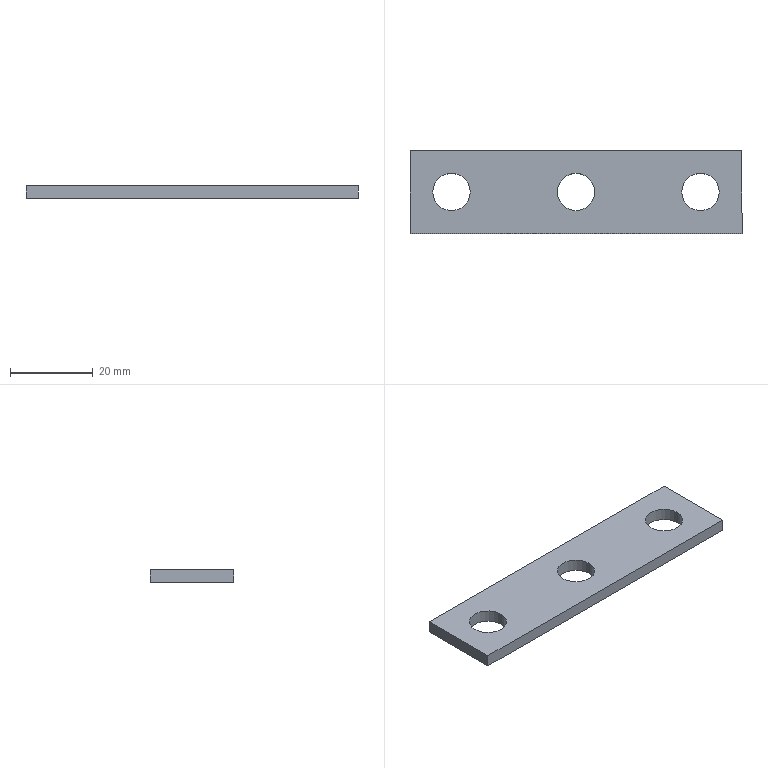Part | SolidWorks | features BaseBody 1 | 1 solid | 12 faces | box 80 x 20 x 3 mm | volume 4227 mm3 | cylinder 6 | plane 6 | commonest cylinder face diameters 9 x6
STEP:
#1=CARTESIAN_POINT('',(-34.5,0.,-3.));
#2=VERTEX_POINT('',#1);
#3=CARTESIAN_POINT('',(-34.5,0.,0.));
#4=VERTEX_POINT('',#3);
#5=CARTESIAN_POINT('',(-34.5,0.,-10.));
#6=DIRECTION('',(0.,0.,1.));
#7=VECTOR('',#6,1000.);
#8=LINE('',#5,#7);
#9=EDGE_CURVE('',#2,#4,#8,.T.);
#10=ORIENTED_EDGE('',*,*,#9,.F.);
#11=CARTESIAN_POINT('',(-25.5,0.,-3.));
#12=VERTEX_POINT('',#11);
#13=CARTESIAN_POINT('',(-30.,0.,-3.));
#14=DIRECTION('',(0.,0.,1.));
#15=DIRECTION('',(1.,0.,0.));
#16=AXIS2_PLACEMENT_3D('',#13,#14,#15);
#17=CIRCLE('',#16,4.5);
#18=EDGE_CURVE('',#12,#2,#17,.T.);
#19=ORIENTED_EDGE('',*,*,#18,.F.);
#20=CARTESIAN_POINT('',(-25.5,0.,0.));
#21=VERTEX_POINT('',#20);
#22=CARTESIAN_POINT('',(-25.5,0.,-10.));
#23=DIRECTION('',(0.,0.,1.));
#24=VECTOR('',#23,1000.);
#25=LINE('',#22,#24);
#26=EDGE_CURVE('',#12,#21,#25,.T.);
#27=ORIENTED_EDGE('',*,*,#26,.T.);
#28=CARTESIAN_POINT('',(-30.,0.,0.));
#29=DIRECTION('',(0.,0.,1.));
#30=DIRECTION('',(-1.,0.,0.));
#31=AXIS2_PLACEMENT_3D('',#28,#29,#30);
#32=CIRCLE('',#31,4.5);
#33=EDGE_CURVE('',#21,#4,#32,.T.);
#34=ORIENTED_EDGE('',*,*,#33,.T.);
#35=EDGE_LOOP('',(#10,#19,#27,#34));
#36=FACE_OUTER_BOUND('',#35,.T.);
#37=CARTESIAN_POINT('',(-30.,0.,-10.));
#38=DIRECTION('',(0.,0.,1.));
#39=DIRECTION('',(1.,0.,0.));
#40=AXIS2_PLACEMENT_3D('',#37,#38,#39);
#41=CYLINDRICAL_SURFACE('',#40,4.5);
#42=ADVANCED_FACE('',(#36),#41,.F.);
#43=CARTESIAN_POINT('',(25.5,0.,-3.));
#44=VERTEX_POINT('',#43);
#45=CARTESIAN_POINT('',(25.5,0.,0.));
#46=VERTEX_POINT('',#45);
#47=CARTESIAN_POINT('',(25.5,0.,-10.));
#48=DIRECTION('',(0.,0.,1.));
#49=VECTOR('',#48,1000.);
#50=LINE('',#47,#49);
#51=EDGE_CURVE('',#44,#46,#50,.T.);
#52=ORIENTED_EDGE('',*,*,#51,.F.);
#53=CARTESIAN_POINT('',(34.5,0.,-3.));
#54=VERTEX_POINT('',#53);
#55=CARTESIAN_POINT('',(30.,0.,-3.));
#56=DIRECTION('',(0.,0.,1.));
#57=DIRECTION('',(1.,0.,0.));
#58=AXIS2_PLACEMENT_3D('',#55,#56,#57);
#59=CIRCLE('',#58,4.5);
#60=EDGE_CURVE('',#54,#44,#59,.T.);
#61=ORIENTED_EDGE('',*,*,#60,.F.);
#62=CARTESIAN_POINT('',(34.5,0.,0.));
#63=VERTEX_POINT('',#62);
#64=CARTESIAN_POINT('',(34.5,0.,-10.));
#65=DIRECTION('',(0.,0.,1.));
#66=VECTOR('',#65,1000.);
#67=LINE('',#64,#66);
#68=EDGE_CURVE('',#54,#63,#67,.T.);
#69=ORIENTED_EDGE('',*,*,#68,.T.);
#70=CARTESIAN_POINT('',(30.,0.,0.));
#71=DIRECTION('',(0.,0.,1.));
#72=DIRECTION('',(1.,0.,0.));
#73=AXIS2_PLACEMENT_3D('',#70,#71,#72);
#74=CIRCLE('',#73,4.5);
#75=EDGE_CURVE('',#63,#46,#74,.T.);
#76=ORIENTED_EDGE('',*,*,#75,.T.);
#77=EDGE_LOOP('',(#52,#61,#69,#76));
#78=FACE_OUTER_BOUND('',#77,.T.);
#79=CARTESIAN_POINT('',(30.,0.,-10.));
#80=DIRECTION('',(0.,0.,1.));
#81=DIRECTION('',(1.,0.,0.));
#82=AXIS2_PLACEMENT_3D('',#79,#80,#81);
#83=CYLINDRICAL_SURFACE('',#82,4.5);
#84=ADVANCED_FACE('',(#78),#83,.F.);
#85=CARTESIAN_POINT('',(-4.5,0.,-3.));
#86=VERTEX_POINT('',#85);
#87=CARTESIAN_POINT('',(-4.5,0.,0.));
#88=VERTEX_POINT('',#87);
#89=CARTESIAN_POINT('',(-4.5,0.,-10.));
#90=DIRECTION('',(0.,0.,1.));
#91=VECTOR('',#90,1000.);
#92=LINE('',#89,#91);
#93=EDGE_CURVE('',#86,#88,#92,.T.);
#94=ORIENTED_EDGE('',*,*,#93,.F.);
#95=CARTESIAN_POINT('',(4.5,0.,-3.));
#96=VERTEX_POINT('',#95);
#97=CARTESIAN_POINT('',(0.,0.,-3.));
#98=DIRECTION('',(0.,0.,1.));
#99=DIRECTION('',(1.,0.,0.));
#100=AXIS2_PLACEMENT_3D('',#97,#98,#99);
#101=CIRCLE('',#100,4.5);
#102=EDGE_CURVE('',#96,#86,#101,.T.);
#103=ORIENTED_EDGE('',*,*,#102,.F.);
#104=CARTESIAN_POINT('',(4.5,0.,0.));
#105=VERTEX_POINT('',#104);
#106=CARTESIAN_POINT('',(4.5,0.,-10.));
#107=DIRECTION('',(0.,0.,1.));
#108=VECTOR('',#107,1000.);
#109=LINE('',#106,#108);
#110=EDGE_CURVE('',#96,#105,#109,.T.);
#111=ORIENTED_EDGE('',*,*,#110,.T.);
#112=CARTESIAN_POINT('',(0.,0.,0.));
#113=DIRECTION('',(0.,0.,1.));
#114=DIRECTION('',(1.,0.,0.));
#115=AXIS2_PLACEMENT_3D('',#112,#113,#114);
#116=CIRCLE('',#115,4.5);
#117=EDGE_CURVE('',#105,#88,#116,.T.);
#118=ORIENTED_EDGE('',*,*,#117,.T.);
#119=EDGE_LOOP('',(#94,#103,#111,#118));
#120=FACE_OUTER_BOUND('',#119,.T.);
#121=CARTESIAN_POINT('',(0.,0.,-10.));
#122=DIRECTION('',(0.,0.,1.));
#123=DIRECTION('',(1.,0.,0.));
#124=AXIS2_PLACEMENT_3D('',#121,#122,#123);
#125=CYLINDRICAL_SURFACE('',#124,4.5);
#126=ADVANCED_FACE('',(#120),#125,.F.);
#127=ORIENTED_EDGE('',*,*,#117,.F.);
#128=CARTESIAN_POINT('',(0.,0.,0.));
#129=DIRECTION('',(0.,0.,1.));
#130=DIRECTION('',(1.,0.,0.));
#131=AXIS2_PLACEMENT_3D('',#128,#129,#130);
#132=CIRCLE('',#131,4.5);
#133=EDGE_CURVE('',#88,#105,#132,.T.);
#134=ORIENTED_EDGE('',*,*,#133,.F.);
#135=EDGE_LOOP('',(#127,#134));
#136=FACE_BOUND('',#135,.T.);
#137=ORIENTED_EDGE('',*,*,#75,.F.);
#138=CARTESIAN_POINT('',(30.,0.,0.));
#139=DIRECTION('',(0.,0.,1.));
#140=DIRECTION('',(1.,0.,0.));
#141=AXIS2_PLACEMENT_3D('',#138,#139,#140);
#142=CIRCLE('',#141,4.5);
#143=EDGE_CURVE('',#46,#63,#142,.T.);
#144=ORIENTED_EDGE('',*,*,#143,.F.);
#145=EDGE_LOOP('',(#137,#144));
#146=FACE_BOUND('',#145,.T.);
#147=ORIENTED_EDGE('',*,*,#33,.F.);
#148=CARTESIAN_POINT('',(-30.,0.,0.));
#149=DIRECTION('',(0.,0.,1.));
#150=DIRECTION('',(-1.,0.,0.));
#151=AXIS2_PLACEMENT_3D('',#148,#149,#150);
#152=CIRCLE('',#151,4.5);
#153=EDGE_CURVE('',#4,#21,#152,.T.);
#154=ORIENTED_EDGE('',*,*,#153,.F.);
#155=EDGE_LOOP('',(#147,#154));
#156=FACE_BOUND('',#155,.T.);
#157=CARTESIAN_POINT('',(40.,-10.,0.));
#158=VERTEX_POINT('',#157);
#159=CARTESIAN_POINT('',(40.,10.,0.));
#160=VERTEX_POINT('',#159);
#161=CARTESIAN_POINT('',(40.,10.,0.));
#162=DIRECTION('',(0.,1.,0.));
#163=VECTOR('',#162,1000.);
#164=LINE('',#161,#163);
#165=EDGE_CURVE('',#158,#160,#164,.T.);
#166=ORIENTED_EDGE('',*,*,#165,.T.);
#167=CARTESIAN_POINT('',(-40.,10.,0.));
#168=VERTEX_POINT('',#167);
#169=CARTESIAN_POINT('',(-40.,10.,0.));
#170=DIRECTION('',(-1.,0.,0.));
#171=VECTOR('',#170,1000.);
#172=LINE('',#169,#171);
#173=EDGE_CURVE('',#160,#168,#172,.T.);
#174=ORIENTED_EDGE('',*,*,#173,.T.);
#175=CARTESIAN_POINT('',(-40.,-10.,0.));
#176=VERTEX_POINT('',#175);
#177=CARTESIAN_POINT('',(-40.,10.,0.));
#178=DIRECTION('',(0.,-1.,0.));
#179=VECTOR('',#178,1000.);
#180=LINE('',#177,#179);
#181=EDGE_CURVE('',#168,#176,#180,.T.);
#182=ORIENTED_EDGE('',*,*,#181,.T.);
#183=CARTESIAN_POINT('',(-40.,-10.,0.));
#184=DIRECTION('',(1.,0.,0.));
#185=VECTOR('',#184,1000.);
#186=LINE('',#183,#185);
#187=EDGE_CURVE('',#176,#158,#186,.T.);
#188=ORIENTED_EDGE('',*,*,#187,.T.);
#189=EDGE_LOOP('',(#166,#174,#182,#188));
#190=FACE_OUTER_BOUND('',#189,.T.);
#191=CARTESIAN_POINT('',(0.,0.,0.));
#192=DIRECTION('',(0.,0.,1.));
#193=DIRECTION('',(1.,0.,0.));
#194=AXIS2_PLACEMENT_3D('',#191,#192,#193);
#195=PLANE('',#194);
#196=ADVANCED_FACE('',(#136,#146,#156,#190),#195,.T.);
#197=ORIENTED_EDGE('',*,*,#102,.T.);
#198=CARTESIAN_POINT('',(0.,0.,-3.));
#199=DIRECTION('',(0.,0.,1.));
#200=DIRECTION('',(1.,0.,0.));
#201=AXIS2_PLACEMENT_3D('',#198,#199,#200);
#202=CIRCLE('',#201,4.5);
#203=EDGE_CURVE('',#86,#96,#202,.T.);
#204=ORIENTED_EDGE('',*,*,#203,.T.);
#205=EDGE_LOOP('',(#197,#204));
#206=FACE_BOUND('',#205,.T.);
#207=ORIENTED_EDGE('',*,*,#60,.T.);
#208=CARTESIAN_POINT('',(30.,0.,-3.));
#209=DIRECTION('',(0.,0.,1.));
#210=DIRECTION('',(1.,0.,0.));
#211=AXIS2_PLACEMENT_3D('',#208,#209,#210);
#212=CIRCLE('',#211,4.5);
#213=EDGE_CURVE('',#44,#54,#212,.T.);
#214=ORIENTED_EDGE('',*,*,#213,.T.);
#215=EDGE_LOOP('',(#207,#214));
#216=FACE_BOUND('',#215,.T.);
#217=ORIENTED_EDGE('',*,*,#18,.T.);
#218=CARTESIAN_POINT('',(-30.,0.,-3.));
#219=DIRECTION('',(0.,0.,1.));
#220=DIRECTION('',(1.,0.,0.));
#221=AXIS2_PLACEMENT_3D('',#218,#219,#220);
#222=CIRCLE('',#221,4.5);
#223=EDGE_CURVE('',#2,#12,#222,.T.);
#224=ORIENTED_EDGE('',*,*,#223,.T.);
#225=EDGE_LOOP('',(#217,#224));
#226=FACE_BOUND('',#225,.T.);
#227=CARTESIAN_POINT('',(40.,-10.,-3.));
#228=VERTEX_POINT('',#227);
#229=CARTESIAN_POINT('',(40.,10.,-3.));
#230=VERTEX_POINT('',#229);
#231=CARTESIAN_POINT('',(40.,10.,-3.));
#232=DIRECTION('',(0.,1.,0.));
#233=VECTOR('',#232,1000.);
#234=LINE('',#231,#233);
#235=EDGE_CURVE('',#228,#230,#234,.T.);
#236=ORIENTED_EDGE('',*,*,#235,.F.);
#237=CARTESIAN_POINT('',(-40.,-10.,-3.));
#238=VERTEX_POINT('',#237);
#239=CARTESIAN_POINT('',(-40.,-10.,-3.));
#240=DIRECTION('',(1.,0.,0.));
#241=VECTOR('',#240,1000.);
#242=LINE('',#239,#241);
#243=EDGE_CURVE('',#238,#228,#242,.T.);
#244=ORIENTED_EDGE('',*,*,#243,.F.);
#245=CARTESIAN_POINT('',(-40.,10.,-3.));
#246=VERTEX_POINT('',#245);
#247=CARTESIAN_POINT('',(-40.,10.,-3.));
#248=DIRECTION('',(0.,-1.,0.));
#249=VECTOR('',#248,1000.);
#250=LINE('',#247,#249);
#251=EDGE_CURVE('',#246,#238,#250,.T.);
#252=ORIENTED_EDGE('',*,*,#251,.F.);
#253=CARTESIAN_POINT('',(-40.,10.,-3.));
#254=DIRECTION('',(-1.,0.,0.));
#255=VECTOR('',#254,1000.);
#256=LINE('',#253,#255);
#257=EDGE_CURVE('',#230,#246,#256,.T.);
#258=ORIENTED_EDGE('',*,*,#257,.F.);
#259=EDGE_LOOP('',(#236,#244,#252,#258));
#260=FACE_OUTER_BOUND('',#259,.T.);
#261=CARTESIAN_POINT('',(0.,0.,-3.));
#262=DIRECTION('',(0.,0.,1.));
#263=DIRECTION('',(1.,0.,0.));
#264=AXIS2_PLACEMENT_3D('',#261,#262,#263);
#265=PLANE('',#264);
#266=ADVANCED_FACE('',(#206,#216,#226,#260),#265,.F.);
#267=ORIENTED_EDGE('',*,*,#173,.F.);
#268=CARTESIAN_POINT('',(40.,10.,-3.));
#269=DIRECTION('',(0.,0.,1.));
#270=VECTOR('',#269,1000.);
#271=LINE('',#268,#270);
#272=EDGE_CURVE('',#230,#160,#271,.T.);
#273=ORIENTED_EDGE('',*,*,#272,.F.);
#274=ORIENTED_EDGE('',*,*,#257,.T.);
#275=CARTESIAN_POINT('',(-40.,10.,-3.));
#276=DIRECTION('',(0.,0.,1.));
#277=VECTOR('',#276,1000.);
#278=LINE('',#275,#277);
#279=EDGE_CURVE('',#246,#168,#278,.T.);
#280=ORIENTED_EDGE('',*,*,#279,.T.);
#281=EDGE_LOOP('',(#267,#273,#274,#280));
#282=FACE_OUTER_BOUND('',#281,.T.);
#283=CARTESIAN_POINT('',(-40.,10.,-3.));
#284=DIRECTION('',(0.,1.,0.));
#285=DIRECTION('',(1.,0.,0.));
#286=AXIS2_PLACEMENT_3D('',#283,#284,#285);
#287=PLANE('',#286);
#288=ADVANCED_FACE('',(#282),#287,.T.);
#289=ORIENTED_EDGE('',*,*,#181,.F.);
#290=ORIENTED_EDGE('',*,*,#279,.F.);
#291=ORIENTED_EDGE('',*,*,#251,.T.);
#292=CARTESIAN_POINT('',(-40.,-10.,-3.));
#293=DIRECTION('',(0.,0.,1.));
#294=VECTOR('',#293,1000.);
#295=LINE('',#292,#294);
#296=EDGE_CURVE('',#238,#176,#295,.T.);
#297=ORIENTED_EDGE('',*,*,#296,.T.);
#298=EDGE_LOOP('',(#289,#290,#291,#297));
#299=FACE_OUTER_BOUND('',#298,.T.);
#300=CARTESIAN_POINT('',(-40.,10.,-3.));
#301=DIRECTION('',(-1.,0.,0.));
#302=DIRECTION('',(0.,0.,1.));
#303=AXIS2_PLACEMENT_3D('',#300,#301,#302);
#304=PLANE('',#303);
#305=ADVANCED_FACE('',(#299),#304,.T.);
#306=ORIENTED_EDGE('',*,*,#187,.F.);
#307=ORIENTED_EDGE('',*,*,#296,.F.);
#308=ORIENTED_EDGE('',*,*,#243,.T.);
#309=CARTESIAN_POINT('',(40.,-10.,-3.));
#310=DIRECTION('',(0.,0.,1.));
#311=VECTOR('',#310,1000.);
#312=LINE('',#309,#311);
#313=EDGE_CURVE('',#228,#158,#312,.T.);
#314=ORIENTED_EDGE('',*,*,#313,.T.);
#315=EDGE_LOOP('',(#306,#307,#308,#314));
#316=FACE_OUTER_BOUND('',#315,.T.);
#317=CARTESIAN_POINT('',(-40.,-10.,-3.));
#318=DIRECTION('',(0.,-1.,0.));
#319=DIRECTION('',(0.,0.,-1.));
#320=AXIS2_PLACEMENT_3D('',#317,#318,#319);
#321=PLANE('',#320);
#322=ADVANCED_FACE('',(#316),#321,.T.);
#323=ORIENTED_EDGE('',*,*,#165,.F.);
#324=ORIENTED_EDGE('',*,*,#313,.F.);
#325=ORIENTED_EDGE('',*,*,#235,.T.);
#326=ORIENTED_EDGE('',*,*,#272,.T.);
#327=EDGE_LOOP('',(#323,#324,#325,#326));
#328=FACE_OUTER_BOUND('',#327,.T.);
#329=CARTESIAN_POINT('',(40.,10.,-3.));
#330=DIRECTION('',(1.,0.,0.));
#331=DIRECTION('',(0.,1.,0.));
#332=AXIS2_PLACEMENT_3D('',#329,#330,#331);
#333=PLANE('',#332);
#334=ADVANCED_FACE('',(#328),#333,.T.);
#335=ORIENTED_EDGE('',*,*,#203,.F.);
#336=ORIENTED_EDGE('',*,*,#93,.T.);
#337=ORIENTED_EDGE('',*,*,#133,.T.);
#338=ORIENTED_EDGE('',*,*,#110,.F.);
#339=EDGE_LOOP('',(#335,#336,#337,#338));
#340=FACE_OUTER_BOUND('',#339,.T.);
#341=CARTESIAN_POINT('',(0.,0.,-10.));
#342=DIRECTION('',(0.,0.,1.));
#343=DIRECTION('',(1.,0.,0.));
#344=AXIS2_PLACEMENT_3D('',#341,#342,#343);
#345=CYLINDRICAL_SURFACE('',#344,4.5);
#346=ADVANCED_FACE('',(#340),#345,.F.);
#347=ORIENTED_EDGE('',*,*,#213,.F.);
#348=ORIENTED_EDGE('',*,*,#51,.T.);
#349=ORIENTED_EDGE('',*,*,#143,.T.);
#350=ORIENTED_EDGE('',*,*,#68,.F.);
#351=EDGE_LOOP('',(#347,#348,#349,#350));
#352=FACE_OUTER_BOUND('',#351,.T.);
#353=CARTESIAN_POINT('',(30.,0.,-10.));
#354=DIRECTION('',(0.,0.,1.));
#355=DIRECTION('',(1.,0.,0.));
#356=AXIS2_PLACEMENT_3D('',#353,#354,#355);
#357=CYLINDRICAL_SURFACE('',#356,4.5);
#358=ADVANCED_FACE('',(#352),#357,.F.);
#359=ORIENTED_EDGE('',*,*,#223,.F.);
#360=ORIENTED_EDGE('',*,*,#9,.T.);
#361=ORIENTED_EDGE('',*,*,#153,.T.);
#362=ORIENTED_EDGE('',*,*,#26,.F.);
#363=EDGE_LOOP('',(#359,#360,#361,#362));
#364=FACE_OUTER_BOUND('',#363,.T.);
#365=CARTESIAN_POINT('',(-30.,0.,-10.));
#366=DIRECTION('',(0.,0.,1.));
#367=DIRECTION('',(1.,0.,0.));
#368=AXIS2_PLACEMENT_3D('',#365,#366,#367);
#369=CYLINDRICAL_SURFACE('',#368,4.5);
#370=ADVANCED_FACE('',(#364),#369,.F.);
#371=CLOSED_SHELL('',(#42,#84,#126,#196,#266,#288,#305,#322,#334,#346,#358,#370));
#372=MANIFOLD_SOLID_BREP('',#371);
#373=CARTESIAN_POINT('',(0.,0.,0.));
#374=DIRECTION('',(0.,0.,1.));
#375=DIRECTION('',(1.,0.,0.));
#376=AXIS2_PLACEMENT_3D('',#373,#374,#375);
#377=(LENGTH_UNIT()NAMED_UNIT(*)SI_UNIT(.MILLI.,.METRE.));
#378=UNCERTAINTY_MEASURE_WITH_UNIT(LENGTH_MEASURE(0.00001),#377,'','');
#379=(NAMED_UNIT(*)PLANE_ANGLE_UNIT()SI_UNIT($,.RADIAN.));
#380=(NAMED_UNIT(*)SI_UNIT($,.STERADIAN.)SOLID_ANGLE_UNIT());
#381=(GEOMETRIC_REPRESENTATION_CONTEXT(3)GLOBAL_UNCERTAINTY_ASSIGNED_CONTEXT((#378))GLOBAL_UNIT_ASSIGNED_CONTEXT((#377,#379,#380))REPRESENTATION_CONTEXT('',''));
#382=ADVANCED_BREP_SHAPE_REPRESENTATION('',(#372,#376),#381);